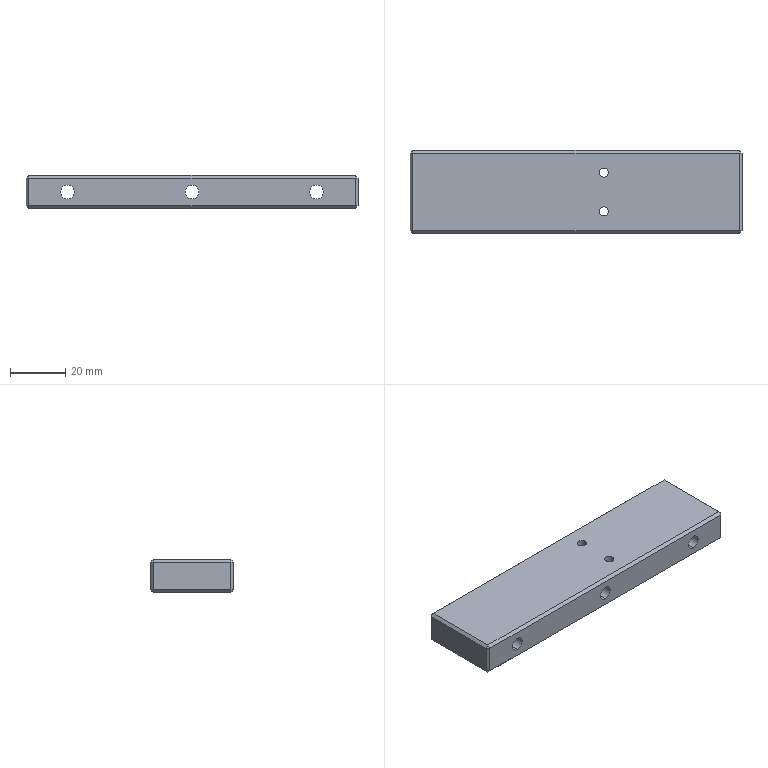Part | STEP file | 03-22 support plate | 1 solid | 36 faces | box 120 x 30 x 12 mm | volume 40909 mm3 | plane 26 | cylinder 10 | commonest cylinder face diameters 5 x6 3.3 x4
STEP:
#1=CARTESIAN_POINT('',(11.65,7.,12.));
#2=VERTEX_POINT('',#1);
#3=CARTESIAN_POINT('',(8.35,7.,12.));
#4=VERTEX_POINT('',#3);
#5=CARTESIAN_POINT('',(10.,7.,12.));
#6=DIRECTION('',(0.,0.,-1.));
#7=DIRECTION('',(-1.,0.,0.));
#8=AXIS2_PLACEMENT_3D('',#5,#6,#7);
#9=CIRCLE('',#8,1.65);
#10=EDGE_CURVE('',#2,#4,#9,.T.);
#11=ORIENTED_EDGE('',*,*,#10,.F.);
#12=CARTESIAN_POINT('',(11.65,7.,0.));
#13=VERTEX_POINT('',#12);
#14=CARTESIAN_POINT('',(11.65,7.,0.));
#15=DIRECTION('',(0.,0.,-1.));
#16=VECTOR('',#15,1000.);
#17=LINE('',#14,#16);
#18=EDGE_CURVE('',#2,#13,#17,.T.);
#19=ORIENTED_EDGE('',*,*,#18,.T.);
#20=CARTESIAN_POINT('',(8.35,7.,0.));
#21=VERTEX_POINT('',#20);
#22=CARTESIAN_POINT('',(10.,7.,0.));
#23=DIRECTION('',(0.,0.,-1.));
#24=DIRECTION('',(-1.,0.,0.));
#25=AXIS2_PLACEMENT_3D('',#22,#23,#24);
#26=CIRCLE('',#25,1.65);
#27=EDGE_CURVE('',#13,#21,#26,.T.);
#28=ORIENTED_EDGE('',*,*,#27,.T.);
#29=CARTESIAN_POINT('',(8.35,7.,0.));
#30=DIRECTION('',(0.,0.,-1.));
#31=VECTOR('',#30,1000.);
#32=LINE('',#29,#31);
#33=EDGE_CURVE('',#4,#21,#32,.T.);
#34=ORIENTED_EDGE('',*,*,#33,.F.);
#35=EDGE_LOOP('',(#11,#19,#28,#34));
#36=FACE_OUTER_BOUND('',#35,.T.);
#37=CARTESIAN_POINT('',(10.,7.,0.));
#38=DIRECTION('',(0.,0.,-1.));
#39=DIRECTION('',(-1.,0.,0.));
#40=AXIS2_PLACEMENT_3D('',#37,#38,#39);
#41=CYLINDRICAL_SURFACE('',#40,1.65);
#42=ADVANCED_FACE('',(#36),#41,.F.);
#43=CARTESIAN_POINT('',(11.65,-7.,12.));
#44=VERTEX_POINT('',#43);
#45=CARTESIAN_POINT('',(8.35,-7.,12.));
#46=VERTEX_POINT('',#45);
#47=CARTESIAN_POINT('',(10.,-7.,12.));
#48=DIRECTION('',(0.,0.,-1.));
#49=DIRECTION('',(-1.,0.,0.));
#50=AXIS2_PLACEMENT_3D('',#47,#48,#49);
#51=CIRCLE('',#50,1.65);
#52=EDGE_CURVE('',#44,#46,#51,.T.);
#53=ORIENTED_EDGE('',*,*,#52,.F.);
#54=CARTESIAN_POINT('',(11.65,-7.,0.));
#55=VERTEX_POINT('',#54);
#56=CARTESIAN_POINT('',(11.65,-7.,0.));
#57=DIRECTION('',(0.,0.,-1.));
#58=VECTOR('',#57,1000.);
#59=LINE('',#56,#58);
#60=EDGE_CURVE('',#44,#55,#59,.T.);
#61=ORIENTED_EDGE('',*,*,#60,.T.);
#62=CARTESIAN_POINT('',(8.35,-7.,0.));
#63=VERTEX_POINT('',#62);
#64=CARTESIAN_POINT('',(10.,-7.,0.));
#65=DIRECTION('',(0.,0.,-1.));
#66=DIRECTION('',(-1.,0.,0.));
#67=AXIS2_PLACEMENT_3D('',#64,#65,#66);
#68=CIRCLE('',#67,1.65);
#69=EDGE_CURVE('',#55,#63,#68,.T.);
#70=ORIENTED_EDGE('',*,*,#69,.T.);
#71=CARTESIAN_POINT('',(8.35,-7.,0.));
#72=DIRECTION('',(0.,0.,-1.));
#73=VECTOR('',#72,1000.);
#74=LINE('',#71,#73);
#75=EDGE_CURVE('',#46,#63,#74,.T.);
#76=ORIENTED_EDGE('',*,*,#75,.F.);
#77=EDGE_LOOP('',(#53,#61,#70,#76));
#78=FACE_OUTER_BOUND('',#77,.T.);
#79=CARTESIAN_POINT('',(10.,-7.,0.));
#80=DIRECTION('',(0.,0.,-1.));
#81=DIRECTION('',(-1.,0.,0.));
#82=AXIS2_PLACEMENT_3D('',#79,#80,#81);
#83=CYLINDRICAL_SURFACE('',#82,1.65);
#84=ADVANCED_FACE('',(#78),#83,.F.);
#85=CARTESIAN_POINT('',(45.,15.,3.5));
#86=VERTEX_POINT('',#85);
#87=CARTESIAN_POINT('',(45.,15.,8.5));
#88=VERTEX_POINT('',#87);
#89=CARTESIAN_POINT('',(45.,15.,6.));
#90=DIRECTION('',(0.,1.,0.));
#91=DIRECTION('',(0.,0.,1.));
#92=AXIS2_PLACEMENT_3D('',#89,#90,#91);
#93=CIRCLE('',#92,2.5);
#94=EDGE_CURVE('',#86,#88,#93,.T.);
#95=ORIENTED_EDGE('',*,*,#94,.T.);
#96=CARTESIAN_POINT('',(45.,-15.,8.5));
#97=VERTEX_POINT('',#96);
#98=CARTESIAN_POINT('',(45.,-15.,8.5));
#99=DIRECTION('',(0.,-1.,0.));
#100=VECTOR('',#99,1000.);
#101=LINE('',#98,#100);
#102=EDGE_CURVE('',#88,#97,#101,.T.);
#103=ORIENTED_EDGE('',*,*,#102,.T.);
#104=CARTESIAN_POINT('',(45.,-15.,3.5));
#105=VERTEX_POINT('',#104);
#106=CARTESIAN_POINT('',(45.,-15.,6.));
#107=DIRECTION('',(0.,-1.,0.));
#108=DIRECTION('',(0.,0.,-1.));
#109=AXIS2_PLACEMENT_3D('',#106,#107,#108);
#110=CIRCLE('',#109,2.5);
#111=EDGE_CURVE('',#97,#105,#110,.T.);
#112=ORIENTED_EDGE('',*,*,#111,.T.);
#113=CARTESIAN_POINT('',(45.,-15.,3.5));
#114=DIRECTION('',(0.,-1.,0.));
#115=VECTOR('',#114,1000.);
#116=LINE('',#113,#115);
#117=EDGE_CURVE('',#86,#105,#116,.T.);
#118=ORIENTED_EDGE('',*,*,#117,.F.);
#119=EDGE_LOOP('',(#95,#103,#112,#118));
#120=FACE_OUTER_BOUND('',#119,.T.);
#121=CARTESIAN_POINT('',(45.,-15.,6.));
#122=DIRECTION('',(0.,-1.,0.));
#123=DIRECTION('',(0.,0.,-1.));
#124=AXIS2_PLACEMENT_3D('',#121,#122,#123);
#125=CYLINDRICAL_SURFACE('',#124,2.5);
#126=ADVANCED_FACE('',(#120),#125,.F.);
#127=CARTESIAN_POINT('',(0.,15.,3.5));
#128=VERTEX_POINT('',#127);
#129=CARTESIAN_POINT('',(0.,15.,8.5));
#130=VERTEX_POINT('',#129);
#131=CARTESIAN_POINT('',(0.,15.,6.));
#132=DIRECTION('',(0.,1.,0.));
#133=DIRECTION('',(0.,0.,1.));
#134=AXIS2_PLACEMENT_3D('',#131,#132,#133);
#135=CIRCLE('',#134,2.5);
#136=EDGE_CURVE('',#128,#130,#135,.T.);
#137=ORIENTED_EDGE('',*,*,#136,.T.);
#138=CARTESIAN_POINT('',(0.,-15.,8.5));
#139=VERTEX_POINT('',#138);
#140=CARTESIAN_POINT('',(0.,-15.,8.5));
#141=DIRECTION('',(0.,-1.,0.));
#142=VECTOR('',#141,1000.);
#143=LINE('',#140,#142);
#144=EDGE_CURVE('',#130,#139,#143,.T.);
#145=ORIENTED_EDGE('',*,*,#144,.T.);
#146=CARTESIAN_POINT('',(0.,-15.,3.5));
#147=VERTEX_POINT('',#146);
#148=CARTESIAN_POINT('',(0.,-15.,6.));
#149=DIRECTION('',(0.,-1.,0.));
#150=DIRECTION('',(0.,0.,-1.));
#151=AXIS2_PLACEMENT_3D('',#148,#149,#150);
#152=CIRCLE('',#151,2.5);
#153=EDGE_CURVE('',#139,#147,#152,.T.);
#154=ORIENTED_EDGE('',*,*,#153,.T.);
#155=CARTESIAN_POINT('',(0.,-15.,3.5));
#156=DIRECTION('',(0.,-1.,0.));
#157=VECTOR('',#156,1000.);
#158=LINE('',#155,#157);
#159=EDGE_CURVE('',#128,#147,#158,.T.);
#160=ORIENTED_EDGE('',*,*,#159,.F.);
#161=EDGE_LOOP('',(#137,#145,#154,#160));
#162=FACE_OUTER_BOUND('',#161,.T.);
#163=CARTESIAN_POINT('',(0.,-15.,6.));
#164=DIRECTION('',(0.,-1.,0.));
#165=DIRECTION('',(0.,0.,-1.));
#166=AXIS2_PLACEMENT_3D('',#163,#164,#165);
#167=CYLINDRICAL_SURFACE('',#166,2.5);
#168=ADVANCED_FACE('',(#162),#167,.F.);
#169=CARTESIAN_POINT('',(-45.,15.,3.5));
#170=VERTEX_POINT('',#169);
#171=CARTESIAN_POINT('',(-45.,15.,8.5));
#172=VERTEX_POINT('',#171);
#173=CARTESIAN_POINT('',(-45.,15.,6.));
#174=DIRECTION('',(0.,1.,0.));
#175=DIRECTION('',(0.,0.,1.));
#176=AXIS2_PLACEMENT_3D('',#173,#174,#175);
#177=CIRCLE('',#176,2.5);
#178=EDGE_CURVE('',#170,#172,#177,.T.);
#179=ORIENTED_EDGE('',*,*,#178,.T.);
#180=CARTESIAN_POINT('',(-45.,-15.,8.5));
#181=VERTEX_POINT('',#180);
#182=CARTESIAN_POINT('',(-45.,-15.,8.5));
#183=DIRECTION('',(0.,-1.,0.));
#184=VECTOR('',#183,1000.);
#185=LINE('',#182,#184);
#186=EDGE_CURVE('',#172,#181,#185,.T.);
#187=ORIENTED_EDGE('',*,*,#186,.T.);
#188=CARTESIAN_POINT('',(-45.,-15.,3.5));
#189=VERTEX_POINT('',#188);
#190=CARTESIAN_POINT('',(-45.,-15.,6.));
#191=DIRECTION('',(0.,-1.,0.));
#192=DIRECTION('',(0.,0.,-1.));
#193=AXIS2_PLACEMENT_3D('',#190,#191,#192);
#194=CIRCLE('',#193,2.5);
#195=EDGE_CURVE('',#181,#189,#194,.T.);
#196=ORIENTED_EDGE('',*,*,#195,.T.);
#197=CARTESIAN_POINT('',(-45.,-15.,3.5));
#198=DIRECTION('',(0.,-1.,0.));
#199=VECTOR('',#198,1000.);
#200=LINE('',#197,#199);
#201=EDGE_CURVE('',#170,#189,#200,.T.);
#202=ORIENTED_EDGE('',*,*,#201,.F.);
#203=EDGE_LOOP('',(#179,#187,#196,#202));
#204=FACE_OUTER_BOUND('',#203,.T.);
#205=CARTESIAN_POINT('',(-45.,-15.,6.));
#206=DIRECTION('',(0.,-1.,0.));
#207=DIRECTION('',(0.,0.,-1.));
#208=AXIS2_PLACEMENT_3D('',#205,#206,#207);
#209=CYLINDRICAL_SURFACE('',#208,2.5);
#210=ADVANCED_FACE('',(#204),#209,.F.);
#211=CARTESIAN_POINT('',(60.,14.,1.));
#212=VERTEX_POINT('',#211);
#213=CARTESIAN_POINT('',(60.,14.,11.));
#214=VERTEX_POINT('',#213);
#215=CARTESIAN_POINT('',(60.,14.,12.));
#216=DIRECTION('',(0.,0.,1.));
#217=VECTOR('',#216,1000.);
#218=LINE('',#215,#217);
#219=EDGE_CURVE('',#212,#214,#218,.T.);
#220=ORIENTED_EDGE('',*,*,#219,.T.);
#221=CARTESIAN_POINT('',(60.,-14.,11.));
#222=VERTEX_POINT('',#221);
#223=CARTESIAN_POINT('',(60.,-15.,11.));
#224=DIRECTION('',(0.,-1.,0.));
#225=VECTOR('',#224,1000.);
#226=LINE('',#223,#225);
#227=EDGE_CURVE('',#214,#222,#226,.T.);
#228=ORIENTED_EDGE('',*,*,#227,.T.);
#229=CARTESIAN_POINT('',(60.,-14.,1.));
#230=VERTEX_POINT('',#229);
#231=CARTESIAN_POINT('',(60.,-14.,12.));
#232=DIRECTION('',(0.,0.,-1.));
#233=VECTOR('',#232,1000.);
#234=LINE('',#231,#233);
#235=EDGE_CURVE('',#222,#230,#234,.T.);
#236=ORIENTED_EDGE('',*,*,#235,.T.);
#237=CARTESIAN_POINT('',(60.,15.,1.));
#238=DIRECTION('',(0.,1.,0.));
#239=VECTOR('',#238,1000.);
#240=LINE('',#237,#239);
#241=EDGE_CURVE('',#230,#212,#240,.T.);
#242=ORIENTED_EDGE('',*,*,#241,.T.);
#243=EDGE_LOOP('',(#220,#228,#236,#242));
#244=FACE_OUTER_BOUND('',#243,.T.);
#245=CARTESIAN_POINT('',(60.,15.,12.));
#246=DIRECTION('',(-1.,0.,0.));
#247=DIRECTION('',(0.,-1.,0.));
#248=AXIS2_PLACEMENT_3D('',#245,#246,#247);
#249=PLANE('',#248);
#250=ADVANCED_FACE('',(#244),#249,.F.);
#251=ORIENTED_EDGE('',*,*,#178,.F.);
#252=CARTESIAN_POINT('',(-45.,15.,6.));
#253=DIRECTION('',(0.,1.,0.));
#254=DIRECTION('',(0.,0.,1.));
#255=AXIS2_PLACEMENT_3D('',#252,#253,#254);
#256=CIRCLE('',#255,2.5);
#257=EDGE_CURVE('',#172,#170,#256,.T.);
#258=ORIENTED_EDGE('',*,*,#257,.F.);
#259=EDGE_LOOP('',(#251,#258));
#260=FACE_BOUND('',#259,.T.);
#261=ORIENTED_EDGE('',*,*,#136,.F.);
#262=CARTESIAN_POINT('',(0.,15.,6.));
#263=DIRECTION('',(0.,1.,0.));
#264=DIRECTION('',(0.,0.,1.));
#265=AXIS2_PLACEMENT_3D('',#262,#263,#264);
#266=CIRCLE('',#265,2.5);
#267=EDGE_CURVE('',#130,#128,#266,.T.);
#268=ORIENTED_EDGE('',*,*,#267,.F.);
#269=EDGE_LOOP('',(#261,#268));
#270=FACE_BOUND('',#269,.T.);
#271=ORIENTED_EDGE('',*,*,#94,.F.);
#272=CARTESIAN_POINT('',(45.,15.,6.));
#273=DIRECTION('',(0.,1.,0.));
#274=DIRECTION('',(0.,0.,1.));
#275=AXIS2_PLACEMENT_3D('',#272,#273,#274);
#276=CIRCLE('',#275,2.5);
#277=EDGE_CURVE('',#88,#86,#276,.T.);
#278=ORIENTED_EDGE('',*,*,#277,.F.);
#279=EDGE_LOOP('',(#271,#278));
#280=FACE_BOUND('',#279,.T.);
#281=CARTESIAN_POINT('',(-59.,15.,11.));
#282=VERTEX_POINT('',#281);
#283=CARTESIAN_POINT('',(59.,15.,11.));
#284=VERTEX_POINT('',#283);
#285=CARTESIAN_POINT('',(60.,15.,11.));
#286=DIRECTION('',(1.,0.,0.));
#287=VECTOR('',#286,1000.);
#288=LINE('',#285,#287);
#289=EDGE_CURVE('',#282,#284,#288,.T.);
#290=ORIENTED_EDGE('',*,*,#289,.T.);
#291=CARTESIAN_POINT('',(59.,15.,1.));
#292=VERTEX_POINT('',#291);
#293=CARTESIAN_POINT('',(59.,15.,12.));
#294=DIRECTION('',(0.,0.,-1.));
#295=VECTOR('',#294,1000.);
#296=LINE('',#293,#295);
#297=EDGE_CURVE('',#284,#292,#296,.T.);
#298=ORIENTED_EDGE('',*,*,#297,.T.);
#299=CARTESIAN_POINT('',(-59.,15.,1.));
#300=VERTEX_POINT('',#299);
#301=CARTESIAN_POINT('',(-60.,15.,1.));
#302=DIRECTION('',(-1.,0.,0.));
#303=VECTOR('',#302,1000.);
#304=LINE('',#301,#303);
#305=EDGE_CURVE('',#292,#300,#304,.T.);
#306=ORIENTED_EDGE('',*,*,#305,.T.);
#307=CARTESIAN_POINT('',(-59.,15.,12.));
#308=DIRECTION('',(0.,0.,1.));
#309=VECTOR('',#308,1000.);
#310=LINE('',#307,#309);
#311=EDGE_CURVE('',#300,#282,#310,.T.);
#312=ORIENTED_EDGE('',*,*,#311,.T.);
#313=EDGE_LOOP('',(#290,#298,#306,#312));
#314=FACE_OUTER_BOUND('',#313,.T.);
#315=CARTESIAN_POINT('',(-60.,15.,12.));
#316=DIRECTION('',(0.,-1.,0.));
#317=DIRECTION('',(0.,0.,-1.));
#318=AXIS2_PLACEMENT_3D('',#315,#316,#317);
#319=PLANE('',#318);
#320=ADVANCED_FACE('',(#260,#270,#280,#314),#319,.F.);
#321=CARTESIAN_POINT('',(-60.,14.,1.));
#322=VERTEX_POINT('',#321);
#323=CARTESIAN_POINT('',(-60.,-14.,1.));
#324=VERTEX_POINT('',#323);
#325=CARTESIAN_POINT('',(-60.,15.,1.));
#326=DIRECTION('',(0.,-1.,0.));
#327=VECTOR('',#326,1000.);
#328=LINE('',#325,#327);
#329=EDGE_CURVE('',#322,#324,#328,.T.);
#330=ORIENTED_EDGE('',*,*,#329,.T.);
#331=CARTESIAN_POINT('',(-60.,-14.,11.));
#332=VERTEX_POINT('',#331);
#333=CARTESIAN_POINT('',(-60.,-14.,12.));
#334=DIRECTION('',(0.,0.,1.));
#335=VECTOR('',#334,1000.);
#336=LINE('',#333,#335);
#337=EDGE_CURVE('',#324,#332,#336,.T.);
#338=ORIENTED_EDGE('',*,*,#337,.T.);
#339=CARTESIAN_POINT('',(-60.,14.,11.));
#340=VERTEX_POINT('',#339);
#341=CARTESIAN_POINT('',(-60.,15.,11.));
#342=DIRECTION('',(0.,1.,0.));
#343=VECTOR('',#342,1000.);
#344=LINE('',#341,#343);
#345=EDGE_CURVE('',#332,#340,#344,.T.);
#346=ORIENTED_EDGE('',*,*,#345,.T.);
#347=CARTESIAN_POINT('',(-60.,14.,12.));
#348=DIRECTION('',(0.,0.,-1.));
#349=VECTOR('',#348,1000.);
#350=LINE('',#347,#349);
#351=EDGE_CURVE('',#340,#322,#350,.T.);
#352=ORIENTED_EDGE('',*,*,#351,.T.);
#353=EDGE_LOOP('',(#330,#338,#346,#352));
#354=FACE_OUTER_BOUND('',#353,.T.);
#355=CARTESIAN_POINT('',(-60.,15.,12.));
#356=DIRECTION('',(1.,0.,0.));
#357=DIRECTION('',(0.,1.,0.));
#358=AXIS2_PLACEMENT_3D('',#355,#356,#357);
#359=PLANE('',#358);
#360=ADVANCED_FACE('',(#354),#359,.F.);
#361=CARTESIAN_POINT('',(0.,-15.,6.));
#362=DIRECTION('',(0.,-1.,0.));
#363=DIRECTION('',(0.,0.,-1.));
#364=AXIS2_PLACEMENT_3D('',#361,#362,#363);
#365=CIRCLE('',#364,2.5);
#366=EDGE_CURVE('',#147,#139,#365,.T.);
#367=ORIENTED_EDGE('',*,*,#366,.F.);
#368=ORIENTED_EDGE('',*,*,#153,.F.);
#369=EDGE_LOOP('',(#367,#368));
#370=FACE_BOUND('',#369,.T.);
#371=CARTESIAN_POINT('',(-45.,-15.,6.));
#372=DIRECTION('',(0.,-1.,0.));
#373=DIRECTION('',(0.,0.,-1.));
#374=AXIS2_PLACEMENT_3D('',#371,#372,#373);
#375=CIRCLE('',#374,2.5);
#376=EDGE_CURVE('',#189,#181,#375,.T.);
#377=ORIENTED_EDGE('',*,*,#376,.F.);
#378=ORIENTED_EDGE('',*,*,#195,.F.);
#379=EDGE_LOOP('',(#377,#378));
#380=FACE_BOUND('',#379,.T.);
#381=CARTESIAN_POINT('',(-59.,-15.,1.));
#382=VERTEX_POINT('',#381);
#383=CARTESIAN_POINT('',(59.,-15.,1.));
#384=VERTEX_POINT('',#383);
#385=CARTESIAN_POINT('',(-60.,-15.,1.));
#386=DIRECTION('',(1.,0.,0.));
#387=VECTOR('',#386,1000.);
#388=LINE('',#385,#387);
#389=EDGE_CURVE('',#382,#384,#388,.T.);
#390=ORIENTED_EDGE('',*,*,#389,.T.);
#391=CARTESIAN_POINT('',(59.,-15.,11.));
#392=VERTEX_POINT('',#391);
#393=CARTESIAN_POINT('',(59.,-15.,12.));
#394=DIRECTION('',(0.,0.,1.));
#395=VECTOR('',#394,1000.);
#396=LINE('',#393,#395);
#397=EDGE_CURVE('',#384,#392,#396,.T.);
#398=ORIENTED_EDGE('',*,*,#397,.T.);
#399=CARTESIAN_POINT('',(-59.,-15.,11.));
#400=VERTEX_POINT('',#399);
#401=CARTESIAN_POINT('',(-60.,-15.,11.));
#402=DIRECTION('',(-1.,0.,0.));
#403=VECTOR('',#402,1000.);
#404=LINE('',#401,#403);
#405=EDGE_CURVE('',#392,#400,#404,.T.);
#406=ORIENTED_EDGE('',*,*,#405,.T.);
#407=CARTESIAN_POINT('',(-59.,-15.,12.));
#408=DIRECTION('',(0.,0.,-1.));
#409=VECTOR('',#408,1000.);
#410=LINE('',#407,#409);
#411=EDGE_CURVE('',#400,#382,#410,.T.);
#412=ORIENTED_EDGE('',*,*,#411,.T.);
#413=EDGE_LOOP('',(#390,#398,#406,#412));
#414=FACE_OUTER_BOUND('',#413,.T.);
#415=CARTESIAN_POINT('',(45.,-15.,6.));
#416=DIRECTION('',(0.,-1.,0.));
#417=DIRECTION('',(0.,0.,-1.));
#418=AXIS2_PLACEMENT_3D('',#415,#416,#417);
#419=CIRCLE('',#418,2.5);
#420=EDGE_CURVE('',#105,#97,#419,.T.);
#421=ORIENTED_EDGE('',*,*,#420,.F.);
#422=ORIENTED_EDGE('',*,*,#111,.F.);
#423=EDGE_LOOP('',(#421,#422));
#424=FACE_BOUND('',#423,.T.);
#425=CARTESIAN_POINT('',(-60.,-15.,12.));
#426=DIRECTION('',(0.,1.,0.));
#427=DIRECTION('',(0.,0.,1.));
#428=AXIS2_PLACEMENT_3D('',#425,#426,#427);
#429=PLANE('',#428);
#430=ADVANCED_FACE('',(#370,#380,#414,#424),#429,.F.);
#431=CARTESIAN_POINT('',(10.,7.,12.));
#432=DIRECTION('',(0.,0.,-1.));
#433=DIRECTION('',(-1.,0.,0.));
#434=AXIS2_PLACEMENT_3D('',#431,#432,#433);
#435=CIRCLE('',#434,1.65);
#436=EDGE_CURVE('',#4,#2,#435,.T.);
#437=ORIENTED_EDGE('',*,*,#436,.T.);
#438=ORIENTED_EDGE('',*,*,#10,.T.);
#439=EDGE_LOOP('',(#437,#438));
#440=FACE_BOUND('',#439,.T.);
#441=CARTESIAN_POINT('',(10.,-7.,12.));
#442=DIRECTION('',(0.,0.,-1.));
#443=DIRECTION('',(-1.,0.,0.));
#444=AXIS2_PLACEMENT_3D('',#441,#442,#443);
#445=CIRCLE('',#444,1.65);
#446=EDGE_CURVE('',#46,#44,#445,.T.);
#447=ORIENTED_EDGE('',*,*,#446,.T.);
#448=ORIENTED_EDGE('',*,*,#52,.T.);
#449=EDGE_LOOP('',(#447,#448));
#450=FACE_BOUND('',#449,.T.);
#451=CARTESIAN_POINT('',(-59.,-14.,12.));
#452=VERTEX_POINT('',#451);
#453=CARTESIAN_POINT('',(59.,-14.,12.));
#454=VERTEX_POINT('',#453);
#455=CARTESIAN_POINT('',(60.,-14.,12.));
#456=DIRECTION('',(1.,0.,0.));
#457=VECTOR('',#456,1000.);
#458=LINE('',#455,#457);
#459=EDGE_CURVE('',#452,#454,#458,.T.);
#460=ORIENTED_EDGE('',*,*,#459,.T.);
#461=CARTESIAN_POINT('',(59.,14.,12.));
#462=VERTEX_POINT('',#461);
#463=CARTESIAN_POINT('',(59.,15.,12.));
#464=DIRECTION('',(0.,1.,0.));
#465=VECTOR('',#464,1000.);
#466=LINE('',#463,#465);
#467=EDGE_CURVE('',#454,#462,#466,.T.);
#468=ORIENTED_EDGE('',*,*,#467,.T.);
#469=CARTESIAN_POINT('',(-59.,14.,12.));
#470=VERTEX_POINT('',#469);
#471=CARTESIAN_POINT('',(-60.,14.,12.));
#472=DIRECTION('',(-1.,0.,0.));
#473=VECTOR('',#472,1000.);
#474=LINE('',#471,#473);
#475=EDGE_CURVE('',#462,#470,#474,.T.);
#476=ORIENTED_EDGE('',*,*,#475,.T.);
#477=CARTESIAN_POINT('',(-59.,-15.,12.));
#478=DIRECTION('',(0.,-1.,0.));
#479=VECTOR('',#478,1000.);
#480=LINE('',#477,#479);
#481=EDGE_CURVE('',#470,#452,#480,.T.);
#482=ORIENTED_EDGE('',*,*,#481,.T.);
#483=EDGE_LOOP('',(#460,#468,#476,#482));
#484=FACE_OUTER_BOUND('',#483,.T.);
#485=CARTESIAN_POINT('',(60.,-15.,12.));
#486=DIRECTION('',(0.,0.,1.));
#487=DIRECTION('',(1.,0.,0.));
#488=AXIS2_PLACEMENT_3D('',#485,#486,#487);
#489=PLANE('',#488);
#490=ADVANCED_FACE('',(#440,#450,#484),#489,.T.);
#491=CARTESIAN_POINT('',(10.,7.,0.));
#492=DIRECTION('',(0.,0.,-1.));
#493=DIRECTION('',(-1.,0.,0.));
#494=AXIS2_PLACEMENT_3D('',#491,#492,#493);
#495=CIRCLE('',#494,1.65);
#496=EDGE_CURVE('',#21,#13,#495,.T.);
#497=ORIENTED_EDGE('',*,*,#496,.F.);
#498=ORIENTED_EDGE('',*,*,#27,.F.);
#499=EDGE_LOOP('',(#497,#498));
#500=FACE_BOUND('',#499,.T.);
#501=CARTESIAN_POINT('',(10.,-7.,0.));
#502=DIRECTION('',(0.,0.,-1.));
#503=DIRECTION('',(-1.,0.,0.));
#504=AXIS2_PLACEMENT_3D('',#501,#502,#503);
#505=CIRCLE('',#504,1.65);
#506=EDGE_CURVE('',#63,#55,#505,.T.);
#507=ORIENTED_EDGE('',*,*,#506,.F.);
#508=ORIENTED_EDGE('',*,*,#69,.F.);
#509=EDGE_LOOP('',(#507,#508));
#510=FACE_BOUND('',#509,.T.);
#511=CARTESIAN_POINT('',(-59.,14.,0.));
#512=VERTEX_POINT('',#511);
#513=CARTESIAN_POINT('',(59.,14.,0.));
#514=VERTEX_POINT('',#513);
#515=CARTESIAN_POINT('',(60.,14.,0.));
#516=DIRECTION('',(1.,0.,0.));
#517=VECTOR('',#516,1000.);
#518=LINE('',#515,#517);
#519=EDGE_CURVE('',#512,#514,#518,.T.);
#520=ORIENTED_EDGE('',*,*,#519,.T.);
#521=CARTESIAN_POINT('',(59.,-14.,0.));
#522=VERTEX_POINT('',#521);
#523=CARTESIAN_POINT('',(59.,-15.,0.));
#524=DIRECTION('',(0.,-1.,0.));
#525=VECTOR('',#524,1000.);
#526=LINE('',#523,#525);
#527=EDGE_CURVE('',#514,#522,#526,.T.);
#528=ORIENTED_EDGE('',*,*,#527,.T.);
#529=CARTESIAN_POINT('',(-59.,-14.,0.));
#530=VERTEX_POINT('',#529);
#531=CARTESIAN_POINT('',(60.,-14.,0.));
#532=DIRECTION('',(-1.,0.,0.));
#533=VECTOR('',#532,1000.);
#534=LINE('',#531,#533);
#535=EDGE_CURVE('',#522,#530,#534,.T.);
#536=ORIENTED_EDGE('',*,*,#535,.T.);
#537=CARTESIAN_POINT('',(-59.,-15.,0.));
#538=DIRECTION('',(0.,1.,0.));
#539=VECTOR('',#538,1000.);
#540=LINE('',#537,#539);
#541=EDGE_CURVE('',#530,#512,#540,.T.);
#542=ORIENTED_EDGE('',*,*,#541,.T.);
#543=EDGE_LOOP('',(#520,#528,#536,#542));
#544=FACE_OUTER_BOUND('',#543,.T.);
#545=CARTESIAN_POINT('',(60.,-15.,0.));
#546=DIRECTION('',(0.,0.,1.));
#547=DIRECTION('',(1.,0.,0.));
#548=AXIS2_PLACEMENT_3D('',#545,#546,#547);
#549=PLANE('',#548);
#550=ADVANCED_FACE('',(#500,#510,#544),#549,.F.);
#551=CARTESIAN_POINT('',(-59.,-14.,0.));
#552=DIRECTION('',(0.7071,0.,-0.7071));
#553=VECTOR('',#552,1000.);
#554=LINE('',#551,#553);
#555=EDGE_CURVE('',#324,#530,#554,.T.);
#556=ORIENTED_EDGE('',*,*,#555,.F.);
#557=ORIENTED_EDGE('',*,*,#329,.F.);
#558=CARTESIAN_POINT('',(-59.,14.,0.));
#559=DIRECTION('',(-0.7071,0.,0.7071));
#560=VECTOR('',#559,1000.);
#561=LINE('',#558,#560);
#562=EDGE_CURVE('',#512,#322,#561,.T.);
#563=ORIENTED_EDGE('',*,*,#562,.F.);
#564=ORIENTED_EDGE('',*,*,#541,.F.);
#565=EDGE_LOOP('',(#556,#557,#563,#564));
#566=FACE_OUTER_BOUND('',#565,.T.);
#567=CARTESIAN_POINT('',(-60.,15.,1.));
#568=DIRECTION('',(0.7071,0.,0.7071));
#569=DIRECTION('',(0.7071,0.,-0.7071));
#570=AXIS2_PLACEMENT_3D('',#567,#568,#569);
#571=PLANE('',#570);
#572=ADVANCED_FACE('',(#566),#571,.F.);
#573=CARTESIAN_POINT('',(-59.5,-14.5,1.));
#574=DIRECTION('',(0.7071,-0.7071,0.));
#575=VECTOR('',#574,1000.);
#576=LINE('',#573,#575);
#577=EDGE_CURVE('',#324,#382,#576,.T.);
#578=ORIENTED_EDGE('',*,*,#577,.F.);
#579=ORIENTED_EDGE('',*,*,#555,.T.);
#580=CARTESIAN_POINT('',(-59.,-14.,0.));
#581=DIRECTION('',(0.,0.7071,-0.7071));
#582=VECTOR('',#581,1000.);
#583=LINE('',#580,#582);
#584=EDGE_CURVE('',#382,#530,#583,.T.);
#585=ORIENTED_EDGE('',*,*,#584,.F.);
#586=EDGE_LOOP('',(#578,#579,#585));
#587=FACE_OUTER_BOUND('',#586,.T.);
#588=CARTESIAN_POINT('',(-59.,-14.,0.));
#589=DIRECTION('',(-0.5774,-0.5774,-0.5774));
#590=DIRECTION('',(0.,0.7071,-0.7071));
#591=AXIS2_PLACEMENT_3D('',#588,#589,#590);
#592=PLANE('',#591);
#593=ADVANCED_FACE('',(#587),#592,.T.);
#594=CARTESIAN_POINT('',(-59.,14.,0.));
#595=DIRECTION('',(0.,0.7071,0.7071));
#596=VECTOR('',#595,1000.);
#597=LINE('',#594,#596);
#598=EDGE_CURVE('',#512,#300,#597,.T.);
#599=ORIENTED_EDGE('',*,*,#598,.F.);
#600=ORIENTED_EDGE('',*,*,#562,.T.);
#601=CARTESIAN_POINT('',(-59.5,14.5,1.));
#602=DIRECTION('',(-0.7071,-0.7071,0.));
#603=VECTOR('',#602,1000.);
#604=LINE('',#601,#603);
#605=EDGE_CURVE('',#300,#322,#604,.T.);
#606=ORIENTED_EDGE('',*,*,#605,.F.);
#607=EDGE_LOOP('',(#599,#600,#606));
#608=FACE_OUTER_BOUND('',#607,.T.);
#609=CARTESIAN_POINT('',(-59.,14.,0.));
#610=DIRECTION('',(-0.5774,0.5774,-0.5774));
#611=DIRECTION('',(0.,0.7071,0.7071));
#612=AXIS2_PLACEMENT_3D('',#609,#610,#611);
#613=PLANE('',#612);
#614=ADVANCED_FACE('',(#608),#613,.T.);
#615=ORIENTED_EDGE('',*,*,#584,.T.);
#616=ORIENTED_EDGE('',*,*,#535,.F.);
#617=CARTESIAN_POINT('',(59.,-14.,0.));
#618=DIRECTION('',(0.,0.7071,-0.7071));
#619=VECTOR('',#618,1000.);
#620=LINE('',#617,#619);
#621=EDGE_CURVE('',#384,#522,#620,.T.);
#622=ORIENTED_EDGE('',*,*,#621,.F.);
#623=ORIENTED_EDGE('',*,*,#389,.F.);
#624=EDGE_LOOP('',(#615,#616,#622,#623));
#625=FACE_OUTER_BOUND('',#624,.T.);
#626=CARTESIAN_POINT('',(-60.,-15.,1.));
#627=DIRECTION('',(0.,0.7071,0.7071));
#628=DIRECTION('',(0.,-0.7071,0.7071));
#629=AXIS2_PLACEMENT_3D('',#626,#627,#628);
#630=PLANE('',#629);
#631=ADVANCED_FACE('',(#625),#630,.F.);
#632=ORIENTED_EDGE('',*,*,#577,.T.);
#633=ORIENTED_EDGE('',*,*,#411,.F.);
#634=CARTESIAN_POINT('',(-59.,-15.,11.));
#635=DIRECTION('',(0.7071,-0.7071,0.));
#636=VECTOR('',#635,1000.);
#637=LINE('',#634,#636);
#638=EDGE_CURVE('',#332,#400,#637,.T.);
#639=ORIENTED_EDGE('',*,*,#638,.F.);
#640=ORIENTED_EDGE('',*,*,#337,.F.);
#641=EDGE_LOOP('',(#632,#633,#639,#640));
#642=FACE_OUTER_BOUND('',#641,.T.);
#643=CARTESIAN_POINT('',(-59.,-15.,12.));
#644=DIRECTION('',(0.7071,0.7071,0.));
#645=DIRECTION('',(-0.7071,0.7071,0.));
#646=AXIS2_PLACEMENT_3D('',#643,#644,#645);
#647=PLANE('',#646);
#648=ADVANCED_FACE('',(#642),#647,.F.);
#649=CARTESIAN_POINT('',(-59.5,14.,11.5));
#650=DIRECTION('',(0.7071,0.,0.7071));
#651=VECTOR('',#650,1000.);
#652=LINE('',#649,#651);
#653=EDGE_CURVE('',#340,#470,#652,.T.);
#654=ORIENTED_EDGE('',*,*,#653,.F.);
#655=ORIENTED_EDGE('',*,*,#345,.F.);
#656=CARTESIAN_POINT('',(-59.5,-14.,11.5));
#657=DIRECTION('',(-0.7071,0.,-0.7071));
#658=VECTOR('',#657,1000.);
#659=LINE('',#656,#658);
#660=EDGE_CURVE('',#452,#332,#659,.T.);
#661=ORIENTED_EDGE('',*,*,#660,.F.);
#662=ORIENTED_EDGE('',*,*,#481,.F.);
#663=EDGE_LOOP('',(#654,#655,#661,#662));
#664=FACE_OUTER_BOUND('',#663,.T.);
#665=CARTESIAN_POINT('',(-59.,-15.,12.));
#666=DIRECTION('',(-0.7071,0.,0.7071));
#667=DIRECTION('',(0.7071,0.,0.7071));
#668=AXIS2_PLACEMENT_3D('',#665,#666,#667);
#669=PLANE('',#668);
#670=ADVANCED_FACE('',(#664),#669,.T.);
#671=ORIENTED_EDGE('',*,*,#605,.T.);
#672=ORIENTED_EDGE('',*,*,#351,.F.);
#673=CARTESIAN_POINT('',(-59.,15.,11.));
#674=DIRECTION('',(-0.7071,-0.7071,0.));
#675=VECTOR('',#674,1000.);
#676=LINE('',#673,#675);
#677=EDGE_CURVE('',#282,#340,#676,.T.);
#678=ORIENTED_EDGE('',*,*,#677,.F.);
#679=ORIENTED_EDGE('',*,*,#311,.F.);
#680=EDGE_LOOP('',(#671,#672,#678,#679));
#681=FACE_OUTER_BOUND('',#680,.T.);
#682=CARTESIAN_POINT('',(-60.,14.,12.));
#683=DIRECTION('',(0.7071,-0.7071,0.));
#684=DIRECTION('',(0.7071,0.7071,0.));
#685=AXIS2_PLACEMENT_3D('',#682,#683,#684);
#686=PLANE('',#685);
#687=ADVANCED_FACE('',(#681),#686,.F.);
#688=ORIENTED_EDGE('',*,*,#598,.T.);
#689=ORIENTED_EDGE('',*,*,#305,.F.);
#690=CARTESIAN_POINT('',(59.,15.,1.));
#691=DIRECTION('',(0.,0.7071,0.7071));
#692=VECTOR('',#691,1000.);
#693=LINE('',#690,#692);
#694=EDGE_CURVE('',#514,#292,#693,.T.);
#695=ORIENTED_EDGE('',*,*,#694,.F.);
#696=ORIENTED_EDGE('',*,*,#519,.F.);
#697=EDGE_LOOP('',(#688,#689,#695,#696));
#698=FACE_OUTER_BOUND('',#697,.T.);
#699=CARTESIAN_POINT('',(-60.,15.,1.));
#700=DIRECTION('',(0.,-0.7071,0.7071));
#701=DIRECTION('',(0.,-0.7071,-0.7071));
#702=AXIS2_PLACEMENT_3D('',#699,#700,#701);
#703=PLANE('',#702);
#704=ADVANCED_FACE('',(#698),#703,.F.);
#705=CARTESIAN_POINT('',(59.,-14.,0.));
#706=DIRECTION('',(0.7071,0.,0.7071));
#707=VECTOR('',#706,1000.);
#708=LINE('',#705,#707);
#709=EDGE_CURVE('',#522,#230,#708,.T.);
#710=ORIENTED_EDGE('',*,*,#709,.F.);
#711=ORIENTED_EDGE('',*,*,#527,.F.);
#712=CARTESIAN_POINT('',(59.5,14.,0.5));
#713=DIRECTION('',(-0.7071,0.,-0.7071));
#714=VECTOR('',#713,1000.);
#715=LINE('',#712,#714);
#716=EDGE_CURVE('',#212,#514,#715,.T.);
#717=ORIENTED_EDGE('',*,*,#716,.F.);
#718=ORIENTED_EDGE('',*,*,#241,.F.);
#719=EDGE_LOOP('',(#710,#711,#717,#718));
#720=FACE_OUTER_BOUND('',#719,.T.);
#721=CARTESIAN_POINT('',(60.,15.,1.));
#722=DIRECTION('',(-0.7071,0.,0.7071));
#723=DIRECTION('',(0.7071,0.,0.7071));
#724=AXIS2_PLACEMENT_3D('',#721,#722,#723);
#725=PLANE('',#724);
#726=ADVANCED_FACE('',(#720),#725,.F.);
#727=ORIENTED_EDGE('',*,*,#621,.T.);
#728=ORIENTED_EDGE('',*,*,#709,.T.);
#729=CARTESIAN_POINT('',(59.5,-14.5,1.));
#730=DIRECTION('',(0.7071,0.7071,0.));
#731=VECTOR('',#730,1000.);
#732=LINE('',#729,#731);
#733=EDGE_CURVE('',#384,#230,#732,.T.);
#734=ORIENTED_EDGE('',*,*,#733,.F.);
#735=EDGE_LOOP('',(#727,#728,#734));
#736=FACE_OUTER_BOUND('',#735,.T.);
#737=CARTESIAN_POINT('',(59.,-14.,0.));
#738=DIRECTION('',(0.5774,-0.5774,-0.5774));
#739=DIRECTION('',(0.7071,0.7071,0.));
#740=AXIS2_PLACEMENT_3D('',#737,#738,#739);
#741=PLANE('',#740);
#742=ADVANCED_FACE('',(#736),#741,.T.);
#743=ORIENTED_EDGE('',*,*,#660,.T.);
#744=ORIENTED_EDGE('',*,*,#638,.T.);
#745=CARTESIAN_POINT('',(-59.,-15.,11.));
#746=DIRECTION('',(0.,-0.7071,-0.7071));
#747=VECTOR('',#746,1000.);
#748=LINE('',#745,#747);
#749=EDGE_CURVE('',#452,#400,#748,.T.);
#750=ORIENTED_EDGE('',*,*,#749,.F.);
#751=EDGE_LOOP('',(#743,#744,#750));
#752=FACE_OUTER_BOUND('',#751,.T.);
#753=CARTESIAN_POINT('',(-59.,-15.,11.));
#754=DIRECTION('',(-0.5774,-0.5774,0.5774));
#755=DIRECTION('',(0.,-0.7071,-0.7071));
#756=AXIS2_PLACEMENT_3D('',#753,#754,#755);
#757=PLANE('',#756);
#758=ADVANCED_FACE('',(#752),#757,.T.);
#759=ORIENTED_EDGE('',*,*,#677,.T.);
#760=ORIENTED_EDGE('',*,*,#653,.T.);
#761=CARTESIAN_POINT('',(-59.,15.,11.));
#762=DIRECTION('',(0.,-0.7071,0.7071));
#763=VECTOR('',#762,1000.);
#764=LINE('',#761,#763);
#765=EDGE_CURVE('',#282,#470,#764,.T.);
#766=ORIENTED_EDGE('',*,*,#765,.F.);
#767=EDGE_LOOP('',(#759,#760,#766));
#768=FACE_OUTER_BOUND('',#767,.T.);
#769=CARTESIAN_POINT('',(-59.,15.,11.));
#770=DIRECTION('',(-0.5774,0.5774,0.5774));
#771=DIRECTION('',(0.,-0.7071,0.7071));
#772=AXIS2_PLACEMENT_3D('',#769,#770,#771);
#773=PLANE('',#772);
#774=ADVANCED_FACE('',(#768),#773,.T.);
#775=ORIENTED_EDGE('',*,*,#716,.T.);
#776=ORIENTED_EDGE('',*,*,#694,.T.);
#777=CARTESIAN_POINT('',(59.,15.,1.));
#778=DIRECTION('',(-0.7071,0.7071,0.));
#779=VECTOR('',#778,1000.);
#780=LINE('',#777,#779);
#781=EDGE_CURVE('',#212,#292,#780,.T.);
#782=ORIENTED_EDGE('',*,*,#781,.F.);
#783=EDGE_LOOP('',(#775,#776,#782));
#784=FACE_OUTER_BOUND('',#783,.T.);
#785=CARTESIAN_POINT('',(59.,15.,1.));
#786=DIRECTION('',(0.5774,0.5774,-0.5774));
#787=DIRECTION('',(-0.7071,0.7071,0.));
#788=AXIS2_PLACEMENT_3D('',#785,#786,#787);
#789=PLANE('',#788);
#790=ADVANCED_FACE('',(#784),#789,.T.);
#791=ORIENTED_EDGE('',*,*,#733,.T.);
#792=ORIENTED_EDGE('',*,*,#235,.F.);
#793=CARTESIAN_POINT('',(60.,-14.,11.));
#794=DIRECTION('',(0.7071,0.7071,0.));
#795=VECTOR('',#794,1000.);
#796=LINE('',#793,#795);
#797=EDGE_CURVE('',#392,#222,#796,.T.);
#798=ORIENTED_EDGE('',*,*,#797,.F.);
#799=ORIENTED_EDGE('',*,*,#397,.F.);
#800=EDGE_LOOP('',(#791,#792,#798,#799));
#801=FACE_OUTER_BOUND('',#800,.T.);
#802=CARTESIAN_POINT('',(60.,-14.,12.));
#803=DIRECTION('',(-0.7071,0.7071,0.));
#804=DIRECTION('',(-0.7071,-0.7071,0.));
#805=AXIS2_PLACEMENT_3D('',#802,#803,#804);
#806=PLANE('',#805);
#807=ADVANCED_FACE('',(#801),#806,.F.);
#808=ORIENTED_EDGE('',*,*,#749,.T.);
#809=ORIENTED_EDGE('',*,*,#405,.F.);
#810=CARTESIAN_POINT('',(59.,-14.5,11.5));
#811=DIRECTION('',(0.,-0.7071,-0.7071));
#812=VECTOR('',#811,1000.);
#813=LINE('',#810,#812);
#814=EDGE_CURVE('',#454,#392,#813,.T.);
#815=ORIENTED_EDGE('',*,*,#814,.F.);
#816=ORIENTED_EDGE('',*,*,#459,.F.);
#817=EDGE_LOOP('',(#808,#809,#815,#816));
#818=FACE_OUTER_BOUND('',#817,.T.);
#819=CARTESIAN_POINT('',(60.,-14.,12.));
#820=DIRECTION('',(0.,-0.7071,0.7071));
#821=DIRECTION('',(0.,-0.7071,-0.7071));
#822=AXIS2_PLACEMENT_3D('',#819,#820,#821);
#823=PLANE('',#822);
#824=ADVANCED_FACE('',(#818),#823,.T.);
#825=ORIENTED_EDGE('',*,*,#765,.T.);
#826=ORIENTED_EDGE('',*,*,#475,.F.);
#827=CARTESIAN_POINT('',(59.,14.,12.));
#828=DIRECTION('',(0.,-0.7071,0.7071));
#829=VECTOR('',#828,1000.);
#830=LINE('',#827,#829);
#831=EDGE_CURVE('',#284,#462,#830,.T.);
#832=ORIENTED_EDGE('',*,*,#831,.F.);
#833=ORIENTED_EDGE('',*,*,#289,.F.);
#834=EDGE_LOOP('',(#825,#826,#832,#833));
#835=FACE_OUTER_BOUND('',#834,.T.);
#836=CARTESIAN_POINT('',(60.,14.,12.));
#837=DIRECTION('',(0.,0.7071,0.7071));
#838=DIRECTION('',(0.,-0.7071,0.7071));
#839=AXIS2_PLACEMENT_3D('',#836,#837,#838);
#840=PLANE('',#839);
#841=ADVANCED_FACE('',(#835),#840,.T.);
#842=ORIENTED_EDGE('',*,*,#781,.T.);
#843=ORIENTED_EDGE('',*,*,#297,.F.);
#844=CARTESIAN_POINT('',(59.5,14.5,11.));
#845=DIRECTION('',(-0.7071,0.7071,0.));
#846=VECTOR('',#845,1000.);
#847=LINE('',#844,#846);
#848=EDGE_CURVE('',#214,#284,#847,.T.);
#849=ORIENTED_EDGE('',*,*,#848,.F.);
#850=ORIENTED_EDGE('',*,*,#219,.F.);
#851=EDGE_LOOP('',(#842,#843,#849,#850));
#852=FACE_OUTER_BOUND('',#851,.T.);
#853=CARTESIAN_POINT('',(59.,15.,12.));
#854=DIRECTION('',(-0.7071,-0.7071,0.));
#855=DIRECTION('',(0.7071,-0.7071,0.));
#856=AXIS2_PLACEMENT_3D('',#853,#854,#855);
#857=PLANE('',#856);
#858=ADVANCED_FACE('',(#852),#857,.F.);
#859=ORIENTED_EDGE('',*,*,#814,.T.);
#860=ORIENTED_EDGE('',*,*,#797,.T.);
#861=CARTESIAN_POINT('',(60.,-14.,11.));
#862=DIRECTION('',(0.7071,0.,-0.7071));
#863=VECTOR('',#862,1000.);
#864=LINE('',#861,#863);
#865=EDGE_CURVE('',#454,#222,#864,.T.);
#866=ORIENTED_EDGE('',*,*,#865,.F.);
#867=EDGE_LOOP('',(#859,#860,#866));
#868=FACE_OUTER_BOUND('',#867,.T.);
#869=CARTESIAN_POINT('',(60.,-14.,11.));
#870=DIRECTION('',(0.5774,-0.5774,0.5774));
#871=DIRECTION('',(0.7071,0.,-0.7071));
#872=AXIS2_PLACEMENT_3D('',#869,#870,#871);
#873=PLANE('',#872);
#874=ADVANCED_FACE('',(#868),#873,.T.);
#875=ORIENTED_EDGE('',*,*,#848,.T.);
#876=ORIENTED_EDGE('',*,*,#831,.T.);
#877=CARTESIAN_POINT('',(59.,14.,12.));
#878=DIRECTION('',(-0.7071,0.,0.7071));
#879=VECTOR('',#878,1000.);
#880=LINE('',#877,#879);
#881=EDGE_CURVE('',#214,#462,#880,.T.);
#882=ORIENTED_EDGE('',*,*,#881,.F.);
#883=EDGE_LOOP('',(#875,#876,#882));
#884=FACE_OUTER_BOUND('',#883,.T.);
#885=CARTESIAN_POINT('',(59.,14.,12.));
#886=DIRECTION('',(0.5774,0.5774,0.5774));
#887=DIRECTION('',(0.,-0.7071,0.7071));
#888=AXIS2_PLACEMENT_3D('',#885,#886,#887);
#889=PLANE('',#888);
#890=ADVANCED_FACE('',(#884),#889,.T.);
#891=ORIENTED_EDGE('',*,*,#865,.T.);
#892=ORIENTED_EDGE('',*,*,#227,.F.);
#893=ORIENTED_EDGE('',*,*,#881,.T.);
#894=ORIENTED_EDGE('',*,*,#467,.F.);
#895=EDGE_LOOP('',(#891,#892,#893,#894));
#896=FACE_OUTER_BOUND('',#895,.T.);
#897=CARTESIAN_POINT('',(59.,-15.,12.));
#898=DIRECTION('',(0.7071,0.,0.7071));
#899=DIRECTION('',(0.7071,0.,-0.7071));
#900=AXIS2_PLACEMENT_3D('',#897,#898,#899);
#901=PLANE('',#900);
#902=ADVANCED_FACE('',(#896),#901,.T.);
#903=ORIENTED_EDGE('',*,*,#186,.F.);
#904=ORIENTED_EDGE('',*,*,#257,.T.);
#905=ORIENTED_EDGE('',*,*,#201,.T.);
#906=ORIENTED_EDGE('',*,*,#376,.T.);
#907=EDGE_LOOP('',(#903,#904,#905,#906));
#908=FACE_OUTER_BOUND('',#907,.T.);
#909=CARTESIAN_POINT('',(-45.,-15.,6.));
#910=DIRECTION('',(0.,-1.,0.));
#911=DIRECTION('',(0.,0.,-1.));
#912=AXIS2_PLACEMENT_3D('',#909,#910,#911);
#913=CYLINDRICAL_SURFACE('',#912,2.5);
#914=ADVANCED_FACE('',(#908),#913,.F.);
#915=ORIENTED_EDGE('',*,*,#144,.F.);
#916=ORIENTED_EDGE('',*,*,#267,.T.);
#917=ORIENTED_EDGE('',*,*,#159,.T.);
#918=ORIENTED_EDGE('',*,*,#366,.T.);
#919=EDGE_LOOP('',(#915,#916,#917,#918));
#920=FACE_OUTER_BOUND('',#919,.T.);
#921=CARTESIAN_POINT('',(0.,-15.,6.));
#922=DIRECTION('',(0.,-1.,0.));
#923=DIRECTION('',(0.,0.,-1.));
#924=AXIS2_PLACEMENT_3D('',#921,#922,#923);
#925=CYLINDRICAL_SURFACE('',#924,2.5);
#926=ADVANCED_FACE('',(#920),#925,.F.);
#927=ORIENTED_EDGE('',*,*,#102,.F.);
#928=ORIENTED_EDGE('',*,*,#277,.T.);
#929=ORIENTED_EDGE('',*,*,#117,.T.);
#930=ORIENTED_EDGE('',*,*,#420,.T.);
#931=EDGE_LOOP('',(#927,#928,#929,#930));
#932=FACE_OUTER_BOUND('',#931,.T.);
#933=CARTESIAN_POINT('',(45.,-15.,6.));
#934=DIRECTION('',(0.,-1.,0.));
#935=DIRECTION('',(0.,0.,-1.));
#936=AXIS2_PLACEMENT_3D('',#933,#934,#935);
#937=CYLINDRICAL_SURFACE('',#936,2.5);
#938=ADVANCED_FACE('',(#932),#937,.F.);
#939=ORIENTED_EDGE('',*,*,#60,.F.);
#940=ORIENTED_EDGE('',*,*,#446,.F.);
#941=ORIENTED_EDGE('',*,*,#75,.T.);
#942=ORIENTED_EDGE('',*,*,#506,.T.);
#943=EDGE_LOOP('',(#939,#940,#941,#942));
#944=FACE_OUTER_BOUND('',#943,.T.);
#945=CARTESIAN_POINT('',(10.,-7.,0.));
#946=DIRECTION('',(0.,0.,-1.));
#947=DIRECTION('',(-1.,0.,0.));
#948=AXIS2_PLACEMENT_3D('',#945,#946,#947);
#949=CYLINDRICAL_SURFACE('',#948,1.65);
#950=ADVANCED_FACE('',(#944),#949,.F.);
#951=ORIENTED_EDGE('',*,*,#18,.F.);
#952=ORIENTED_EDGE('',*,*,#436,.F.);
#953=ORIENTED_EDGE('',*,*,#33,.T.);
#954=ORIENTED_EDGE('',*,*,#496,.T.);
#955=EDGE_LOOP('',(#951,#952,#953,#954));
#956=FACE_OUTER_BOUND('',#955,.T.);
#957=CARTESIAN_POINT('',(10.,7.,0.));
#958=DIRECTION('',(0.,0.,-1.));
#959=DIRECTION('',(-1.,0.,0.));
#960=AXIS2_PLACEMENT_3D('',#957,#958,#959);
#961=CYLINDRICAL_SURFACE('',#960,1.65);
#962=ADVANCED_FACE('',(#956),#961,.F.);
#963=CLOSED_SHELL('',(#42,#84,#126,#168,#210,#250,#320,#360,#430,#490,#550,#572,#593,#614,#631,#648,#670,#687,#704,#726,#742,#758,#774,#790,#807,#824,#841,#858,#874,#890,#902,#914,#926,#938,#950,#962));
#964=MANIFOLD_SOLID_BREP('',#963);
#965=CARTESIAN_POINT('',(0.,0.,0.));
#966=DIRECTION('',(0.,0.,1.));
#967=DIRECTION('',(1.,0.,0.));
#968=AXIS2_PLACEMENT_3D('',#965,#966,#967);
#969=(LENGTH_UNIT()NAMED_UNIT(*)SI_UNIT(.MILLI.,.METRE.));
#970=UNCERTAINTY_MEASURE_WITH_UNIT(LENGTH_MEASURE(0.00001),#969,'','');
#971=(NAMED_UNIT(*)PLANE_ANGLE_UNIT()SI_UNIT($,.RADIAN.));
#972=(NAMED_UNIT(*)SI_UNIT($,.STERADIAN.)SOLID_ANGLE_UNIT());
#973=(GEOMETRIC_REPRESENTATION_CONTEXT(3)GLOBAL_UNCERTAINTY_ASSIGNED_CONTEXT((#970))GLOBAL_UNIT_ASSIGNED_CONTEXT((#969,#971,#972))REPRESENTATION_CONTEXT('',''));
#974=ADVANCED_BREP_SHAPE_REPRESENTATION('',(#964,#968),#973);